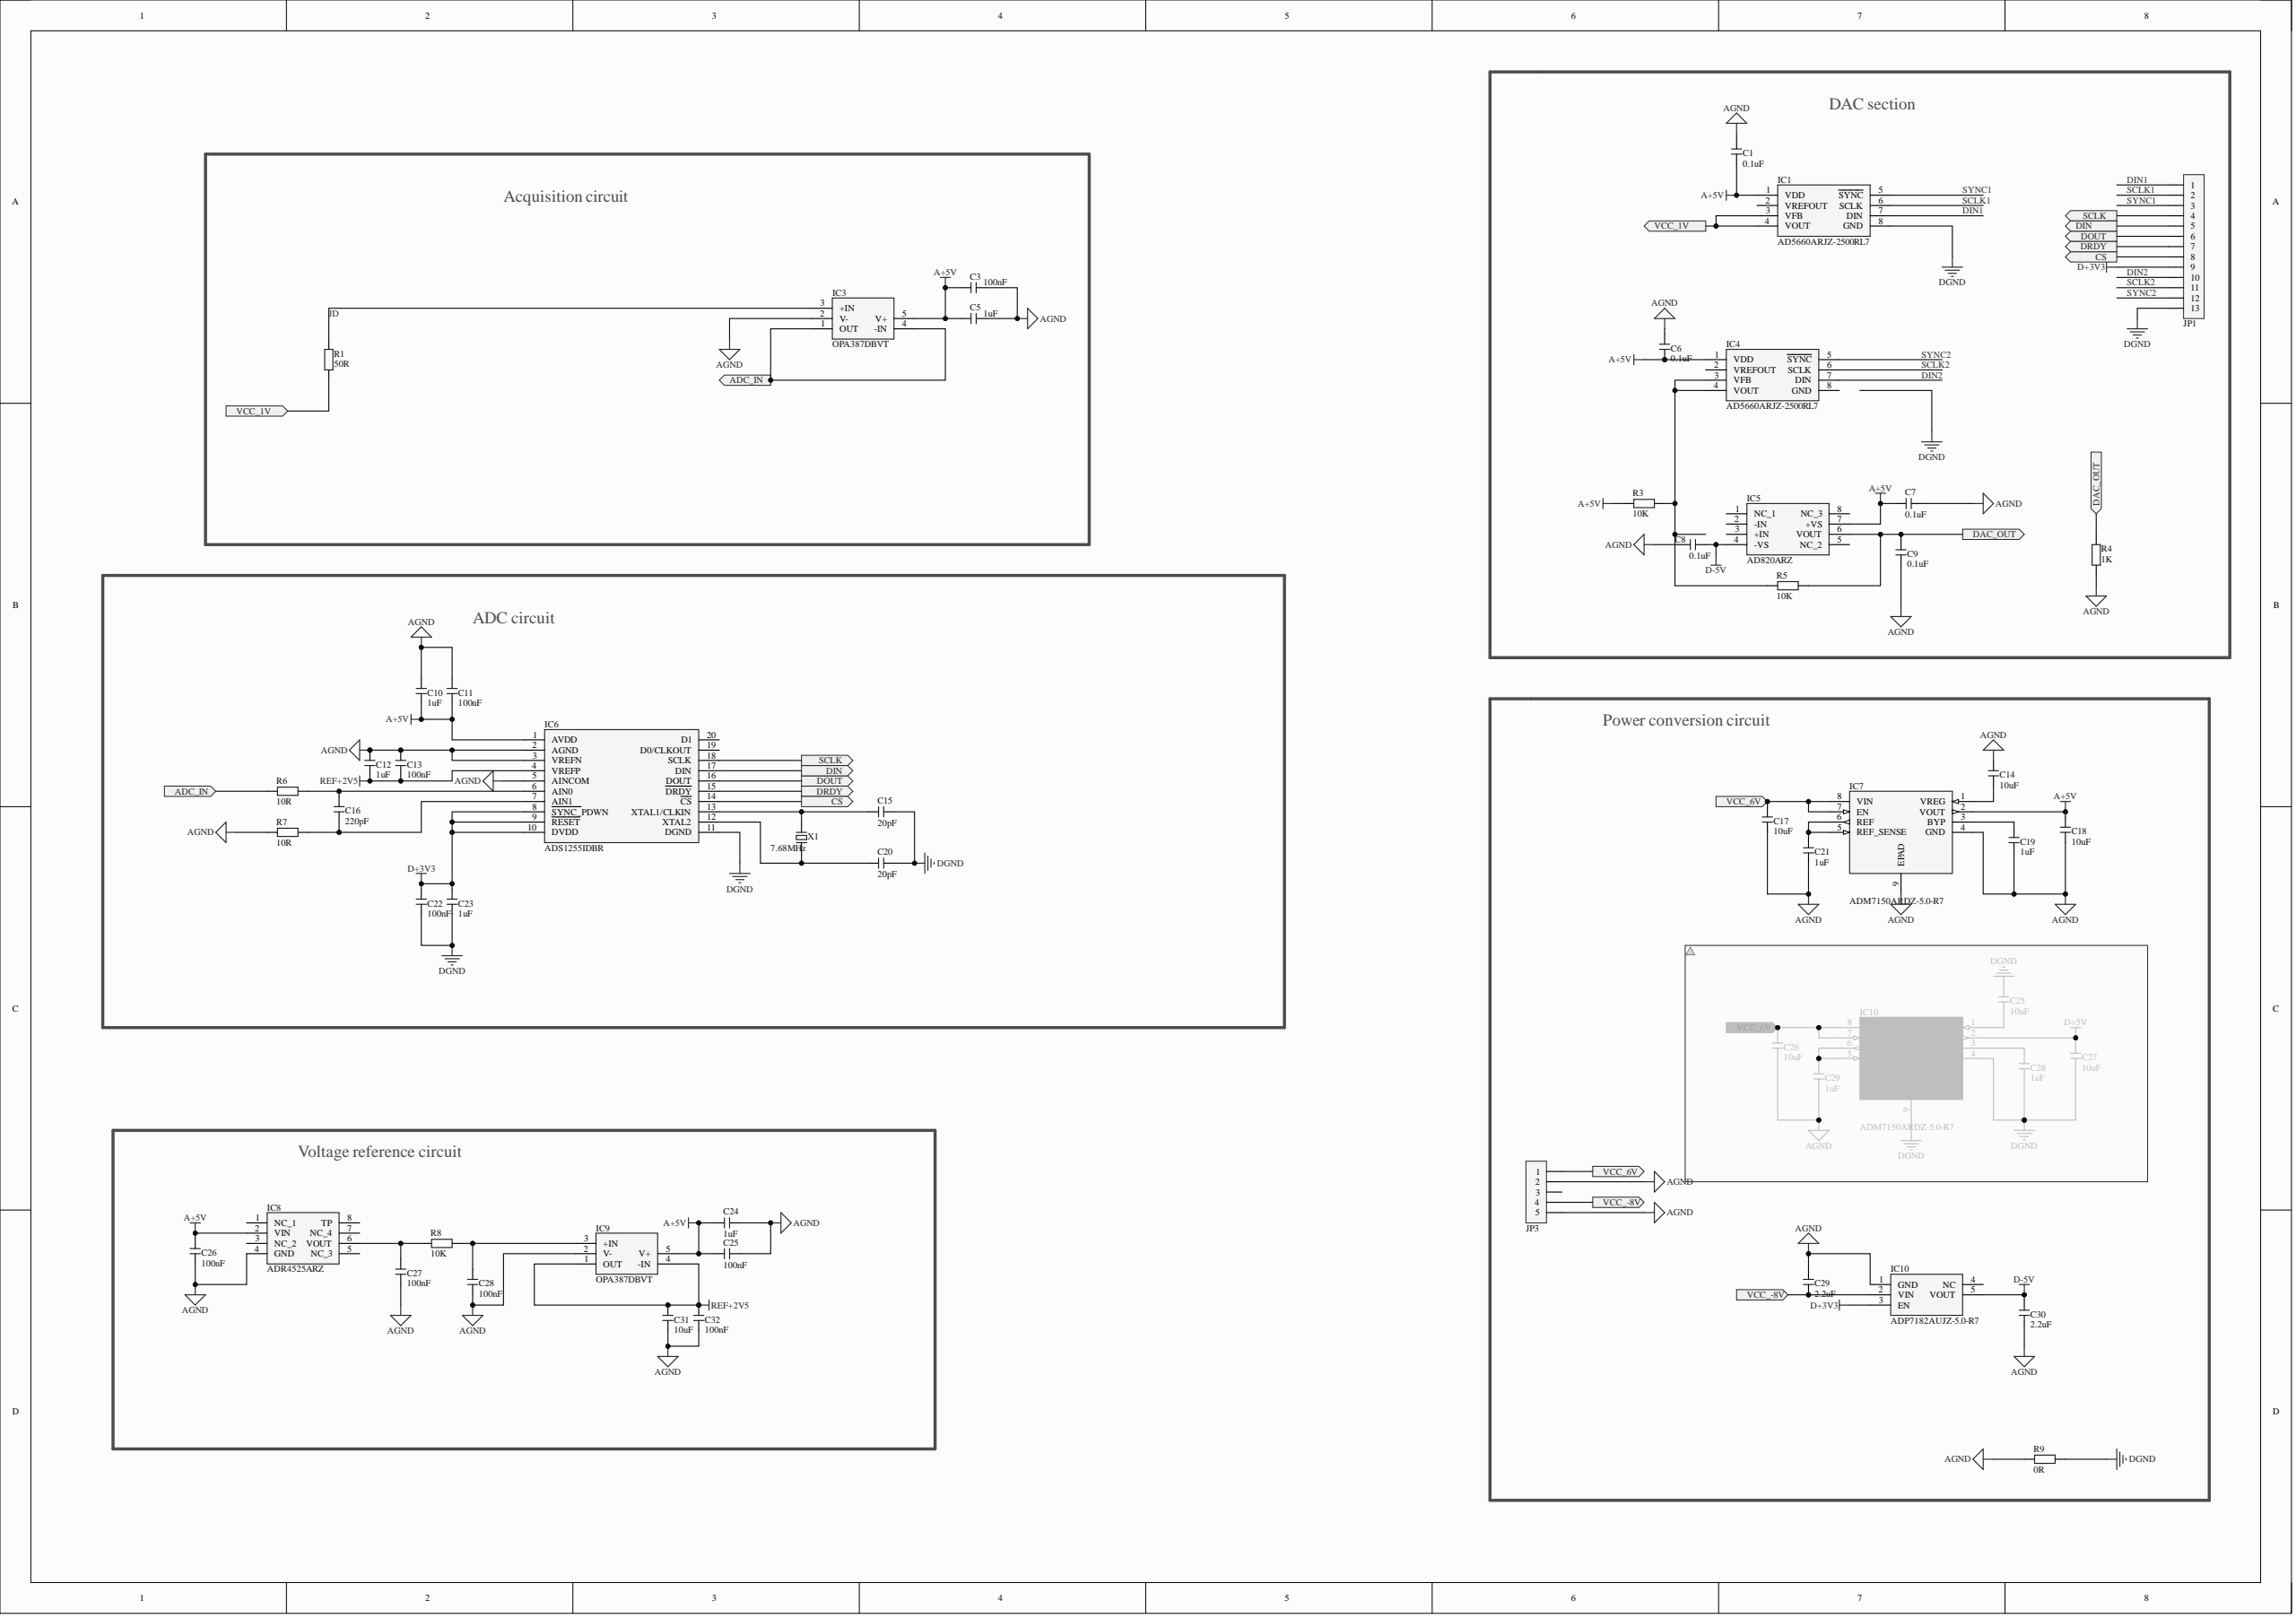Circuit board | Altium Designer | 50 parts | 33 nets
Bill of materials:
Comment,Description,Designator,Footprint,LibRef,Quantity
"0.1uF","Non-polar chip capacitor","C1, C6, C7, C8, C9","C 0603_L","C","5"
"100nF","Non-polar chip capacitor","C3, C11, C13, C22, C25, C26, C27, C28, C32","C 0603_L","C","9"
"1uF","Non-polar chip capacitor","C5, C10, C12, C19, C21, C23, C24","C 0603_L","C","7"
"10uF","Non-polar chip capacitor","C14, C17, C18, C31","C 0603_L","C","4"
"20pF","Non-polar chip capacitor","C15, C20","C 0603_L","C","2"
"220pF","Non-polar chip capacitor","C16","C 0805_L","C","1"
"2.2uF","Non-polar chip capacitor","C29, C30","C 0805_L","C","2"
"AD5660ARJZ-2500RL7","Integrated Circuit","IC1, IC4","SOT65P280X145-8N","AD5620ARJZ-1500RL7, AD5660ARJZ-2500RL7","2"
"OPA387DBVT","Integrated Circuit","IC3","SOT95P280X100-5N","OPA387DBVT","1"
"AD820ARZ","Integrated Circuit","IC5","SOIC127P600X175-8N","AD820ARZ","1"
"ADS1255IDBR","Integrated Circuit","IC6","SOP65P780X200-20N","ADS1255IDBR","1"
"ADM7150ARDZ-5.0-R7","Integrated Circuit","IC7","SOIC127P600X175-9N","ADM7150ARDZ-5.0-R7","1"
"ADR4525ARZ","Integrated Circuit","IC8","SOIC127P600X175-8N","ADR4525ARZ","1"
"OPA387DBVT","Integrated Circuit","IC9","SOT95P280X145-5N","OPA387DBVT","1"
"ADP7182AUJZ-5.0-R7","Integrated Circuit","IC10","SOT95P280X100-5N","ADP7182AUJZ-5.0-R7","1"
"HDR-1X13","13P connector","JP1","HDR2.54-LI-13P","Header 13","1"
"HDR-1X5","5P connector","JP3","HDR2.54-LI-5P","Header 5","1"
"50R","PTFR0603B100RN9","R1","R 0805_L","R","1"
"10K","PTFR0603B100RN9","R3, R5","R 0603_L","R","2"
"1K","Chip resistor","R4","R 0603_L","R","1"
"10R","Chip resistor","R6, R7","R 0603_L","R","2"
"10K","Chip resistor","R8","R 0805_L","R","1"
"0R","Chip resistor","R9","R 0805_L","R","1"
"7.68MHz","2-pin passive crystal oscillator","X1","OSC HC-49SMD","XTAL-2P","1"
Netlist (Protel format):
[
C1
C 0603_L
0.1uF



]
[
C3
C 0603_L
100nF



]
[
C5
C 0603_L
1uF



]
[
C6
C 0603_L
0.1uF



]
[
C7
C 0603_L
0.1uF



]
[
C8
C 0603_L
0.1uF



]
[
C9
C 0603_L
0.1uF



]
[
C10
C 0603_L
1uF



]
[
C11
C 0603_L
100nF



]
[
C12
C 0603_L
1uF



]
[
C13
C 0603_L
100nF



]
[
C14
C 0603_L
10uF



]
[
C15
C 0603_L
20pF



]
[
C16
C 0805_L
220pF



]
[
C17
C 0603_L
10uF



]
[
C18
C 0603_L
10uF



]
[
C19
C 0603_L
1uF



]
[
C20
C 0603_L
20pF



]
[
C21
C 0603_L
1uF



]
[
C22
C 0603_L
100nF



]
[
C23
C 0603_L
1uF



]
[
C24
C 0603_L
1uF



]
[
C25
C 0603_L
100nF



]
[
C26
C 0603_L
100nF



]
[
C27
C 0603_L
100nF



]
[
C28
C 0603_L
100nF



]
[
C29
C 0805_L
2.2uF



]
[
C30
C 0805_L
2.2uF



]
[
C31
C 0603_L
10uF



]
[
C32
C 0603_L
100nF



]
[
IC1
SOT65P280X145-8N
AD5660ARJZ-2500RL7



]
[
IC3
SOT95P280X100-5N
OPA387DBVT



]
[
IC4
SOT65P280X145-8N
AD5660ARJZ-2500RL7



]
[
IC5
SOIC127P600X175-8N
AD820ARZ



]
[
IC6
SOP65P780X200-20N
ADS1255IDBR



]
[
IC7
SOIC127P600X175-9N
ADM7150ARDZ-5.0-R7



]
[
IC8
SOIC127P600X175-8N
ADR4525ARZ



]
[
IC9
SOT95P280X145-5N
OPA387DBVT



]
[
IC10
SOT95P280X100-5N
ADP7182AUJZ-5.0-R7



]
[
JP1
HDR2.54-LI-13P
HDR-1X13



]
[
JP3
HDR2.54-LI-5P
HDR-1X5



]
[
R1
R 0805_L
50R



]
[
R3
R 0603_L
10K



]
[
R4
R 0603_L
1K



]
[
R5
R 0603_L
10K



]
[
R6
R 0603_L
10R



]
[
R7
R 0603_L
10R



]
[
R8
R 0805_L
10K



]
[
R9
R 0805_L
0R



]
[
X1
OSC HC-49SMD
7.68MHz



]
(
SYNC2
IC4-5
JP1-12
)
(
SYNC1
IC1-5
JP1-3
)
(
SCLK2
IC4-6
JP1-11
)
(
SCLK1
IC1-6
JP1-2
)
(
REF+2V5
C12-1
C13-1
C31-2
C32-2
IC6-4
IC9-1
IC9-4
)
(
NetIC6_18
IC6-18
JP1-4
)
(
NetIC6_17
IC6-17
JP1-5
)
(
NetIC6_16
IC6-16
JP1-6
)
(
NetIC6_15
IC6-15
JP1-7
)
(
NetIC6_14
IC6-14
JP1-8
)
(
NetIC4_3
IC4-3
IC4-4
R3-1
R5-2
)
(
NetIC3_1
IC3-1
IC3-4
R6-1
)
(
NetIC1_3
IC1-3
IC1-4
R1-1
)
(
NetC29_2
C29-2
IC10-2
JP3-4
)
(
NetC28_1
C28-1
IC9-3
R8-2
)
(
NetC27_1
C27-1
IC8-6
R8-1
)
(
NetC21_1
C21-1
IC7-5
IC7-6
)
(
NetC20_1
C20-1
IC6-12
X1-1
)
(
NetC19_1
C19-1
IC7-3
)
(
NetC17_1
C17-1
IC7-7
IC7-8
JP3-1
)
(
NetC16_2
C16-2
IC6-6
R6-2
)
(
NetC16_1
C16-1
IC6-7
R7-2
)
(
NetC15_1
C15-1
IC6-13
X1-2
)
(
NetC14_1
C14-1
IC7-1
)
(
NetC9_1
C9-1
IC5-6
R4-2
R5-1
)
(
JD
IC3-3
R1-2
)
(
DIN2
IC4-7
JP1-10
)
(
DIN1
IC1-7
JP1-1
)
(
DGND
C15-2
C20-2
C22-2
C23-2
IC1-8
IC6-11
JP1-13
R9-2
)
(
D-5V
C8-2
C30-1
IC5-4
IC10-5
)
(
D+3V3
C22-1
C23-1
IC6-8
IC6-9
IC6-10
IC10-3
JP1-9
)
(
AGND
C1-2
C3-2
C5-2
C6-2
C7-2
C8-1
C9-2
C10-2
C11-2
C12-2
C13-2
C14-2
C17-2
C18-2
C19-2
C21-2
C24-2
C25-2
C26-2
C27-2
C28-2
C29-1
C30-2
C31-1
C32-1
IC3-2
IC6-2
IC6-3
IC6-5
IC7-4
IC7-9
IC8-4
IC9-2
IC10-1
JP3-2
JP3-5
R4-1
R7-1
R9-1
)
(
A+5V
C1-1
C3-1
C5-1
C6-1
C7-1
C10-1
C11-1
C18-1
C24-1
C25-1
C26-1
IC1-1
IC3-5
IC4-1
IC5-7
IC6-1
IC7-2
IC8-2
IC9-5
R3-2
)